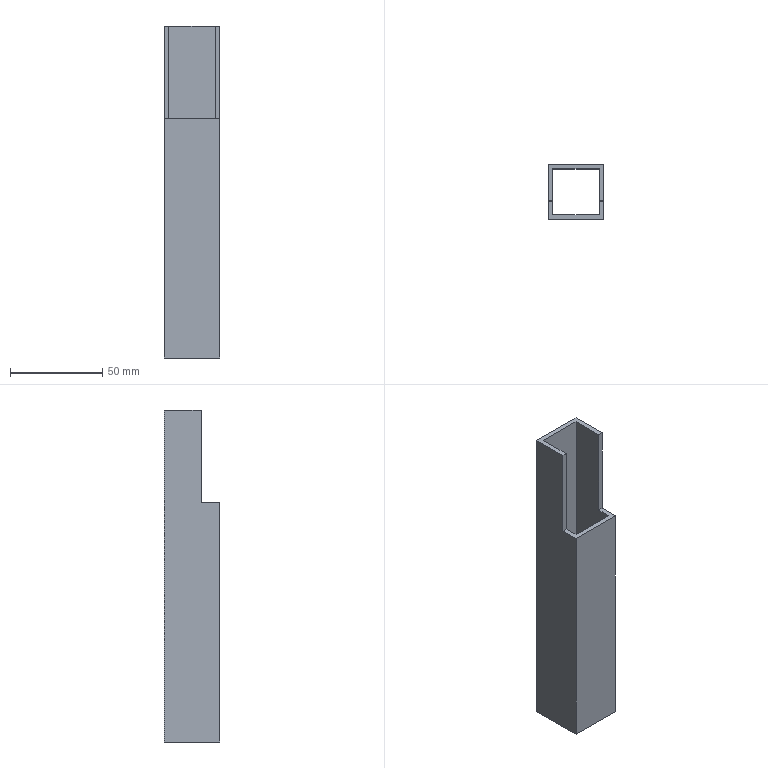Part | SolidWorks | features ICE 2, Extrusion 1 | 1 solid | 13 faces | box 30 x 30 x 180 mm | volume 43875 mm3 | plane 13
STEP:
#1=CARTESIAN_POINT('',(15.,-5.,130.));
#2=VERTEX_POINT('',#1);
#3=CARTESIAN_POINT('',(15.,-5.,180.));
#4=VERTEX_POINT('',#3);
#5=CARTESIAN_POINT('',(15.,-5.,180.));
#6=DIRECTION('',(0.,0.,1.));
#7=VECTOR('',#6,1000.);
#8=LINE('',#5,#7);
#9=EDGE_CURVE('',#2,#4,#8,.T.);
#10=ORIENTED_EDGE('',*,*,#9,.F.);
#11=CARTESIAN_POINT('',(15.,-15.,130.));
#12=VERTEX_POINT('',#11);
#13=CARTESIAN_POINT('',(15.,-283.666,130.));
#14=DIRECTION('',(0.,1.,0.));
#15=VECTOR('',#14,1000.);
#16=LINE('',#13,#15);
#17=EDGE_CURVE('',#12,#2,#16,.T.);
#18=ORIENTED_EDGE('',*,*,#17,.F.);
#19=CARTESIAN_POINT('',(15.,-15.,0.));
#20=VERTEX_POINT('',#19);
#21=CARTESIAN_POINT('',(15.,-15.,180.));
#22=DIRECTION('',(0.,0.,-1.));
#23=VECTOR('',#22,1000.);
#24=LINE('',#21,#23);
#25=EDGE_CURVE('',#12,#20,#24,.T.);
#26=ORIENTED_EDGE('',*,*,#25,.T.);
#27=CARTESIAN_POINT('',(15.,15.,0.));
#28=VERTEX_POINT('',#27);
#29=CARTESIAN_POINT('',(15.,15.,0.));
#30=DIRECTION('',(0.,1.,0.));
#31=VECTOR('',#30,1000.);
#32=LINE('',#29,#31);
#33=EDGE_CURVE('',#20,#28,#32,.T.);
#34=ORIENTED_EDGE('',*,*,#33,.T.);
#35=CARTESIAN_POINT('',(15.,15.,180.));
#36=VERTEX_POINT('',#35);
#37=CARTESIAN_POINT('',(15.,15.,180.));
#38=DIRECTION('',(0.,0.,-1.));
#39=VECTOR('',#38,1000.);
#40=LINE('',#37,#39);
#41=EDGE_CURVE('',#36,#28,#40,.T.);
#42=ORIENTED_EDGE('',*,*,#41,.F.);
#43=CARTESIAN_POINT('',(15.,15.,180.));
#44=DIRECTION('',(0.,1.,0.));
#45=VECTOR('',#44,1000.);
#46=LINE('',#43,#45);
#47=EDGE_CURVE('',#4,#36,#46,.T.);
#48=ORIENTED_EDGE('',*,*,#47,.F.);
#49=EDGE_LOOP('',(#10,#18,#26,#34,#42,#48));
#50=FACE_OUTER_BOUND('',#49,.T.);
#51=CARTESIAN_POINT('',(15.,15.,180.));
#52=DIRECTION('',(-1.,0.,0.));
#53=DIRECTION('',(0.,0.,1.));
#54=AXIS2_PLACEMENT_3D('',#51,#52,#53);
#55=PLANE('',#54);
#56=ADVANCED_FACE('',(#50),#55,.F.);
#57=CARTESIAN_POINT('',(-15.,-15.,130.));
#58=VERTEX_POINT('',#57);
#59=CARTESIAN_POINT('',(-15.,-15.,130.));
#60=DIRECTION('',(1.,0.,0.));
#61=VECTOR('',#60,1000.);
#62=LINE('',#59,#61);
#63=EDGE_CURVE('',#58,#12,#62,.T.);
#64=ORIENTED_EDGE('',*,*,#63,.F.);
#65=CARTESIAN_POINT('',(-15.,-15.,0.));
#66=VERTEX_POINT('',#65);
#67=CARTESIAN_POINT('',(-15.,-15.,180.));
#68=DIRECTION('',(0.,0.,-1.));
#69=VECTOR('',#68,1000.);
#70=LINE('',#67,#69);
#71=EDGE_CURVE('',#58,#66,#70,.T.);
#72=ORIENTED_EDGE('',*,*,#71,.T.);
#73=CARTESIAN_POINT('',(-15.,-15.,0.));
#74=DIRECTION('',(1.,0.,0.));
#75=VECTOR('',#74,1000.);
#76=LINE('',#73,#75);
#77=EDGE_CURVE('',#66,#20,#76,.T.);
#78=ORIENTED_EDGE('',*,*,#77,.T.);
#79=ORIENTED_EDGE('',*,*,#25,.F.);
#80=EDGE_LOOP('',(#64,#72,#78,#79));
#81=FACE_OUTER_BOUND('',#80,.T.);
#82=CARTESIAN_POINT('',(-15.,-15.,180.));
#83=DIRECTION('',(0.,1.,0.));
#84=DIRECTION('',(0.,0.,1.));
#85=AXIS2_PLACEMENT_3D('',#82,#83,#84);
#86=PLANE('',#85);
#87=ADVANCED_FACE('',(#81),#86,.F.);
#88=CARTESIAN_POINT('',(-15.,15.,180.));
#89=VERTEX_POINT('',#88);
#90=CARTESIAN_POINT('',(-15.,-5.,180.));
#91=VERTEX_POINT('',#90);
#92=CARTESIAN_POINT('',(-15.,15.,180.));
#93=DIRECTION('',(0.,-1.,0.));
#94=VECTOR('',#93,1000.);
#95=LINE('',#92,#94);
#96=EDGE_CURVE('',#89,#91,#95,.T.);
#97=ORIENTED_EDGE('',*,*,#96,.T.);
#98=CARTESIAN_POINT('',(-12.5,-5.,180.));
#99=VERTEX_POINT('',#98);
#100=CARTESIAN_POINT('',(-15.,-5.,180.));
#101=DIRECTION('',(1.,0.,0.));
#102=VECTOR('',#101,1000.);
#103=LINE('',#100,#102);
#104=EDGE_CURVE('',#91,#99,#103,.T.);
#105=ORIENTED_EDGE('',*,*,#104,.T.);
#106=CARTESIAN_POINT('',(-12.5,12.5,180.));
#107=VERTEX_POINT('',#106);
#108=CARTESIAN_POINT('',(-12.5,12.5,180.));
#109=DIRECTION('',(0.,1.,0.));
#110=VECTOR('',#109,1000.);
#111=LINE('',#108,#110);
#112=EDGE_CURVE('',#99,#107,#111,.T.);
#113=ORIENTED_EDGE('',*,*,#112,.T.);
#114=CARTESIAN_POINT('',(12.5,12.5,180.));
#115=VERTEX_POINT('',#114);
#116=CARTESIAN_POINT('',(12.5,12.5,180.));
#117=DIRECTION('',(1.,0.,0.));
#118=VECTOR('',#117,1000.);
#119=LINE('',#116,#118);
#120=EDGE_CURVE('',#107,#115,#119,.T.);
#121=ORIENTED_EDGE('',*,*,#120,.T.);
#122=CARTESIAN_POINT('',(12.5,-5.,180.));
#123=VERTEX_POINT('',#122);
#124=CARTESIAN_POINT('',(12.5,12.5,180.));
#125=DIRECTION('',(0.,-1.,0.));
#126=VECTOR('',#125,1000.);
#127=LINE('',#124,#126);
#128=EDGE_CURVE('',#115,#123,#127,.T.);
#129=ORIENTED_EDGE('',*,*,#128,.T.);
#130=CARTESIAN_POINT('',(-15.,-5.,180.));
#131=DIRECTION('',(1.,0.,0.));
#132=VECTOR('',#131,1000.);
#133=LINE('',#130,#132);
#134=EDGE_CURVE('',#123,#4,#133,.T.);
#135=ORIENTED_EDGE('',*,*,#134,.T.);
#136=ORIENTED_EDGE('',*,*,#47,.T.);
#137=CARTESIAN_POINT('',(-15.,15.,180.));
#138=DIRECTION('',(-1.,0.,0.));
#139=VECTOR('',#138,1000.);
#140=LINE('',#137,#139);
#141=EDGE_CURVE('',#36,#89,#140,.T.);
#142=ORIENTED_EDGE('',*,*,#141,.T.);
#143=EDGE_LOOP('',(#97,#105,#113,#121,#129,#135,#136,#142));
#144=FACE_OUTER_BOUND('',#143,.T.);
#145=CARTESIAN_POINT('',(0.,0.,180.));
#146=DIRECTION('',(0.,0.,1.));
#147=DIRECTION('',(1.,0.,0.));
#148=AXIS2_PLACEMENT_3D('',#145,#146,#147);
#149=PLANE('',#148);
#150=ADVANCED_FACE('',(#144),#149,.T.);
#151=CARTESIAN_POINT('',(-15.,15.,0.));
#152=VERTEX_POINT('',#151);
#153=CARTESIAN_POINT('',(-15.,15.,0.));
#154=DIRECTION('',(-1.,0.,0.));
#155=VECTOR('',#154,1000.);
#156=LINE('',#153,#155);
#157=EDGE_CURVE('',#28,#152,#156,.T.);
#158=ORIENTED_EDGE('',*,*,#157,.T.);
#159=CARTESIAN_POINT('',(-15.,15.,180.));
#160=DIRECTION('',(0.,0.,-1.));
#161=VECTOR('',#160,1000.);
#162=LINE('',#159,#161);
#163=EDGE_CURVE('',#89,#152,#162,.T.);
#164=ORIENTED_EDGE('',*,*,#163,.F.);
#165=ORIENTED_EDGE('',*,*,#141,.F.);
#166=ORIENTED_EDGE('',*,*,#41,.T.);
#167=EDGE_LOOP('',(#158,#164,#165,#166));
#168=FACE_OUTER_BOUND('',#167,.T.);
#169=CARTESIAN_POINT('',(-15.,15.,180.));
#170=DIRECTION('',(0.,-1.,0.));
#171=DIRECTION('',(0.,0.,-1.));
#172=AXIS2_PLACEMENT_3D('',#169,#170,#171);
#173=PLANE('',#172);
#174=ADVANCED_FACE('',(#168),#173,.F.);
#175=ORIENTED_EDGE('',*,*,#71,.F.);
#176=CARTESIAN_POINT('',(-15.,-5.,130.));
#177=VERTEX_POINT('',#176);
#178=CARTESIAN_POINT('',(-15.,-283.666,130.));
#179=DIRECTION('',(0.,1.,0.));
#180=VECTOR('',#179,1000.);
#181=LINE('',#178,#180);
#182=EDGE_CURVE('',#58,#177,#181,.T.);
#183=ORIENTED_EDGE('',*,*,#182,.T.);
#184=CARTESIAN_POINT('',(-15.,-5.,180.));
#185=DIRECTION('',(0.,0.,-1.));
#186=VECTOR('',#185,1000.);
#187=LINE('',#184,#186);
#188=EDGE_CURVE('',#91,#177,#187,.T.);
#189=ORIENTED_EDGE('',*,*,#188,.F.);
#190=ORIENTED_EDGE('',*,*,#96,.F.);
#191=ORIENTED_EDGE('',*,*,#163,.T.);
#192=CARTESIAN_POINT('',(-15.,15.,0.));
#193=DIRECTION('',(0.,-1.,0.));
#194=VECTOR('',#193,1000.);
#195=LINE('',#192,#194);
#196=EDGE_CURVE('',#152,#66,#195,.T.);
#197=ORIENTED_EDGE('',*,*,#196,.T.);
#198=EDGE_LOOP('',(#175,#183,#189,#190,#191,#197));
#199=FACE_OUTER_BOUND('',#198,.T.);
#200=CARTESIAN_POINT('',(-15.,15.,180.));
#201=DIRECTION('',(1.,0.,0.));
#202=DIRECTION('',(0.,0.,-1.));
#203=AXIS2_PLACEMENT_3D('',#200,#201,#202);
#204=PLANE('',#203);
#205=ADVANCED_FACE('',(#199),#204,.F.);
#206=CARTESIAN_POINT('',(-12.5,12.5,0.));
#207=VERTEX_POINT('',#206);
#208=CARTESIAN_POINT('',(12.5,12.5,0.));
#209=VERTEX_POINT('',#208);
#210=CARTESIAN_POINT('',(12.5,12.5,0.));
#211=DIRECTION('',(1.,0.,0.));
#212=VECTOR('',#211,1000.);
#213=LINE('',#210,#212);
#214=EDGE_CURVE('',#207,#209,#213,.T.);
#215=ORIENTED_EDGE('',*,*,#214,.F.);
#216=CARTESIAN_POINT('',(-12.5,-12.5,0.));
#217=VERTEX_POINT('',#216);
#218=CARTESIAN_POINT('',(-12.5,12.5,0.));
#219=DIRECTION('',(0.,1.,0.));
#220=VECTOR('',#219,1000.);
#221=LINE('',#218,#220);
#222=EDGE_CURVE('',#217,#207,#221,.T.);
#223=ORIENTED_EDGE('',*,*,#222,.F.);
#224=CARTESIAN_POINT('',(12.5,-12.5,0.));
#225=VERTEX_POINT('',#224);
#226=CARTESIAN_POINT('',(12.5,-12.5,0.));
#227=DIRECTION('',(-1.,0.,0.));
#228=VECTOR('',#227,1000.);
#229=LINE('',#226,#228);
#230=EDGE_CURVE('',#225,#217,#229,.T.);
#231=ORIENTED_EDGE('',*,*,#230,.F.);
#232=CARTESIAN_POINT('',(12.5,12.5,0.));
#233=DIRECTION('',(0.,-1.,0.));
#234=VECTOR('',#233,1000.);
#235=LINE('',#232,#234);
#236=EDGE_CURVE('',#209,#225,#235,.T.);
#237=ORIENTED_EDGE('',*,*,#236,.F.);
#238=EDGE_LOOP('',(#215,#223,#231,#237));
#239=FACE_BOUND('',#238,.T.);
#240=ORIENTED_EDGE('',*,*,#33,.F.);
#241=ORIENTED_EDGE('',*,*,#77,.F.);
#242=ORIENTED_EDGE('',*,*,#196,.F.);
#243=ORIENTED_EDGE('',*,*,#157,.F.);
#244=EDGE_LOOP('',(#240,#241,#242,#243));
#245=FACE_OUTER_BOUND('',#244,.T.);
#246=CARTESIAN_POINT('',(0.,0.,0.));
#247=DIRECTION('',(0.,0.,1.));
#248=DIRECTION('',(1.,0.,0.));
#249=AXIS2_PLACEMENT_3D('',#246,#247,#248);
#250=PLANE('',#249);
#251=ADVANCED_FACE('',(#239,#245),#250,.F.);
#252=CARTESIAN_POINT('',(-12.5,-5.,130.));
#253=VERTEX_POINT('',#252);
#254=CARTESIAN_POINT('',(-12.5,-5.,180.));
#255=DIRECTION('',(0.,0.,-1.));
#256=VECTOR('',#255,1000.);
#257=LINE('',#254,#256);
#258=EDGE_CURVE('',#99,#253,#257,.T.);
#259=ORIENTED_EDGE('',*,*,#258,.T.);
#260=CARTESIAN_POINT('',(-12.5,-12.5,130.));
#261=VERTEX_POINT('',#260);
#262=CARTESIAN_POINT('',(-12.5,12.5,130.));
#263=DIRECTION('',(0.,-1.,0.));
#264=VECTOR('',#263,1000.);
#265=LINE('',#262,#264);
#266=EDGE_CURVE('',#253,#261,#265,.T.);
#267=ORIENTED_EDGE('',*,*,#266,.T.);
#268=CARTESIAN_POINT('',(-12.5,-12.5,180.));
#269=DIRECTION('',(0.,0.,-1.));
#270=VECTOR('',#269,1000.);
#271=LINE('',#268,#270);
#272=EDGE_CURVE('',#261,#217,#271,.T.);
#273=ORIENTED_EDGE('',*,*,#272,.T.);
#274=ORIENTED_EDGE('',*,*,#222,.T.);
#275=CARTESIAN_POINT('',(-12.5,12.5,180.));
#276=DIRECTION('',(0.,0.,-1.));
#277=VECTOR('',#276,1000.);
#278=LINE('',#275,#277);
#279=EDGE_CURVE('',#107,#207,#278,.T.);
#280=ORIENTED_EDGE('',*,*,#279,.F.);
#281=ORIENTED_EDGE('',*,*,#112,.F.);
#282=EDGE_LOOP('',(#259,#267,#273,#274,#280,#281));
#283=FACE_OUTER_BOUND('',#282,.T.);
#284=CARTESIAN_POINT('',(-12.5,12.5,180.));
#285=DIRECTION('',(-1.,0.,0.));
#286=DIRECTION('',(0.,0.,1.));
#287=AXIS2_PLACEMENT_3D('',#284,#285,#286);
#288=PLANE('',#287);
#289=ADVANCED_FACE('',(#283),#288,.F.);
#290=ORIENTED_EDGE('',*,*,#272,.F.);
#291=CARTESIAN_POINT('',(12.5,-12.5,130.));
#292=VERTEX_POINT('',#291);
#293=CARTESIAN_POINT('',(12.5,-12.5,130.));
#294=DIRECTION('',(1.,0.,0.));
#295=VECTOR('',#294,1000.);
#296=LINE('',#293,#295);
#297=EDGE_CURVE('',#261,#292,#296,.T.);
#298=ORIENTED_EDGE('',*,*,#297,.T.);
#299=CARTESIAN_POINT('',(12.5,-12.5,180.));
#300=DIRECTION('',(0.,0.,-1.));
#301=VECTOR('',#300,1000.);
#302=LINE('',#299,#301);
#303=EDGE_CURVE('',#292,#225,#302,.T.);
#304=ORIENTED_EDGE('',*,*,#303,.T.);
#305=ORIENTED_EDGE('',*,*,#230,.T.);
#306=EDGE_LOOP('',(#290,#298,#304,#305));
#307=FACE_OUTER_BOUND('',#306,.T.);
#308=CARTESIAN_POINT('',(12.5,-12.5,180.));
#309=DIRECTION('',(0.,-1.,0.));
#310=DIRECTION('',(0.,0.,-1.));
#311=AXIS2_PLACEMENT_3D('',#308,#309,#310);
#312=PLANE('',#311);
#313=ADVANCED_FACE('',(#307),#312,.F.);
#314=ORIENTED_EDGE('',*,*,#303,.F.);
#315=CARTESIAN_POINT('',(12.5,-5.,130.));
#316=VERTEX_POINT('',#315);
#317=CARTESIAN_POINT('',(12.5,12.5,130.));
#318=DIRECTION('',(0.,1.,0.));
#319=VECTOR('',#318,1000.);
#320=LINE('',#317,#319);
#321=EDGE_CURVE('',#292,#316,#320,.T.);
#322=ORIENTED_EDGE('',*,*,#321,.T.);
#323=CARTESIAN_POINT('',(12.5,-5.,180.));
#324=DIRECTION('',(0.,0.,1.));
#325=VECTOR('',#324,1000.);
#326=LINE('',#323,#325);
#327=EDGE_CURVE('',#316,#123,#326,.T.);
#328=ORIENTED_EDGE('',*,*,#327,.T.);
#329=ORIENTED_EDGE('',*,*,#128,.F.);
#330=CARTESIAN_POINT('',(12.5,12.5,180.));
#331=DIRECTION('',(0.,0.,-1.));
#332=VECTOR('',#331,1000.);
#333=LINE('',#330,#332);
#334=EDGE_CURVE('',#115,#209,#333,.T.);
#335=ORIENTED_EDGE('',*,*,#334,.T.);
#336=ORIENTED_EDGE('',*,*,#236,.T.);
#337=EDGE_LOOP('',(#314,#322,#328,#329,#335,#336));
#338=FACE_OUTER_BOUND('',#337,.T.);
#339=CARTESIAN_POINT('',(12.5,12.5,180.));
#340=DIRECTION('',(1.,0.,0.));
#341=DIRECTION('',(0.,0.,-1.));
#342=AXIS2_PLACEMENT_3D('',#339,#340,#341);
#343=PLANE('',#342);
#344=ADVANCED_FACE('',(#338),#343,.F.);
#345=ORIENTED_EDGE('',*,*,#214,.T.);
#346=ORIENTED_EDGE('',*,*,#334,.F.);
#347=ORIENTED_EDGE('',*,*,#120,.F.);
#348=ORIENTED_EDGE('',*,*,#279,.T.);
#349=EDGE_LOOP('',(#345,#346,#347,#348));
#350=FACE_OUTER_BOUND('',#349,.T.);
#351=CARTESIAN_POINT('',(12.5,12.5,180.));
#352=DIRECTION('',(0.,1.,0.));
#353=DIRECTION('',(0.,0.,1.));
#354=AXIS2_PLACEMENT_3D('',#351,#352,#353);
#355=PLANE('',#354);
#356=ADVANCED_FACE('',(#350),#355,.F.);
#357=ORIENTED_EDGE('',*,*,#266,.F.);
#358=CARTESIAN_POINT('',(-15.,-5.,130.));
#359=DIRECTION('',(1.,0.,0.));
#360=VECTOR('',#359,1000.);
#361=LINE('',#358,#360);
#362=EDGE_CURVE('',#177,#253,#361,.T.);
#363=ORIENTED_EDGE('',*,*,#362,.F.);
#364=ORIENTED_EDGE('',*,*,#182,.F.);
#365=ORIENTED_EDGE('',*,*,#63,.T.);
#366=ORIENTED_EDGE('',*,*,#17,.T.);
#367=CARTESIAN_POINT('',(-15.,-5.,130.));
#368=DIRECTION('',(1.,0.,0.));
#369=VECTOR('',#368,1000.);
#370=LINE('',#367,#369);
#371=EDGE_CURVE('',#316,#2,#370,.T.);
#372=ORIENTED_EDGE('',*,*,#371,.F.);
#373=ORIENTED_EDGE('',*,*,#321,.F.);
#374=ORIENTED_EDGE('',*,*,#297,.F.);
#375=EDGE_LOOP('',(#357,#363,#364,#365,#366,#372,#373,#374));
#376=FACE_OUTER_BOUND('',#375,.T.);
#377=CARTESIAN_POINT('',(-15.,-283.666,130.));
#378=DIRECTION('',(0.,0.,-1.));
#379=DIRECTION('',(-1.,0.,0.));
#380=AXIS2_PLACEMENT_3D('',#377,#378,#379);
#381=PLANE('',#380);
#382=ADVANCED_FACE('',(#376),#381,.F.);
#383=ORIENTED_EDGE('',*,*,#258,.F.);
#384=ORIENTED_EDGE('',*,*,#104,.F.);
#385=ORIENTED_EDGE('',*,*,#188,.T.);
#386=ORIENTED_EDGE('',*,*,#362,.T.);
#387=EDGE_LOOP('',(#383,#384,#385,#386));
#388=FACE_OUTER_BOUND('',#387,.T.);
#389=CARTESIAN_POINT('',(-15.,-5.,180.));
#390=DIRECTION('',(0.,1.,0.));
#391=DIRECTION('',(0.,0.,1.));
#392=AXIS2_PLACEMENT_3D('',#389,#390,#391);
#393=PLANE('',#392);
#394=ADVANCED_FACE('',(#388),#393,.F.);
#395=ORIENTED_EDGE('',*,*,#327,.F.);
#396=ORIENTED_EDGE('',*,*,#371,.T.);
#397=ORIENTED_EDGE('',*,*,#9,.T.);
#398=ORIENTED_EDGE('',*,*,#134,.F.);
#399=EDGE_LOOP('',(#395,#396,#397,#398));
#400=FACE_OUTER_BOUND('',#399,.T.);
#401=CARTESIAN_POINT('',(-15.,-5.,180.));
#402=DIRECTION('',(0.,1.,0.));
#403=DIRECTION('',(0.,0.,1.));
#404=AXIS2_PLACEMENT_3D('',#401,#402,#403);
#405=PLANE('',#404);
#406=ADVANCED_FACE('',(#400),#405,.F.);
#407=CLOSED_SHELL('',(#56,#87,#150,#174,#205,#251,#289,#313,#344,#356,#382,#394,#406));
#408=MANIFOLD_SOLID_BREP('',#407);
#409=CARTESIAN_POINT('',(0.,0.,0.));
#410=DIRECTION('',(0.,0.,1.));
#411=DIRECTION('',(1.,0.,0.));
#412=AXIS2_PLACEMENT_3D('',#409,#410,#411);
#413=(LENGTH_UNIT()NAMED_UNIT(*)SI_UNIT(.MILLI.,.METRE.));
#414=UNCERTAINTY_MEASURE_WITH_UNIT(LENGTH_MEASURE(0.00001),#413,'','');
#415=(NAMED_UNIT(*)PLANE_ANGLE_UNIT()SI_UNIT($,.RADIAN.));
#416=(NAMED_UNIT(*)SI_UNIT($,.STERADIAN.)SOLID_ANGLE_UNIT());
#417=(GEOMETRIC_REPRESENTATION_CONTEXT(3)GLOBAL_UNCERTAINTY_ASSIGNED_CONTEXT((#414))GLOBAL_UNIT_ASSIGNED_CONTEXT((#413,#415,#416))REPRESENTATION_CONTEXT('',''));
#418=ADVANCED_BREP_SHAPE_REPRESENTATION('',(#408,#412),#417);